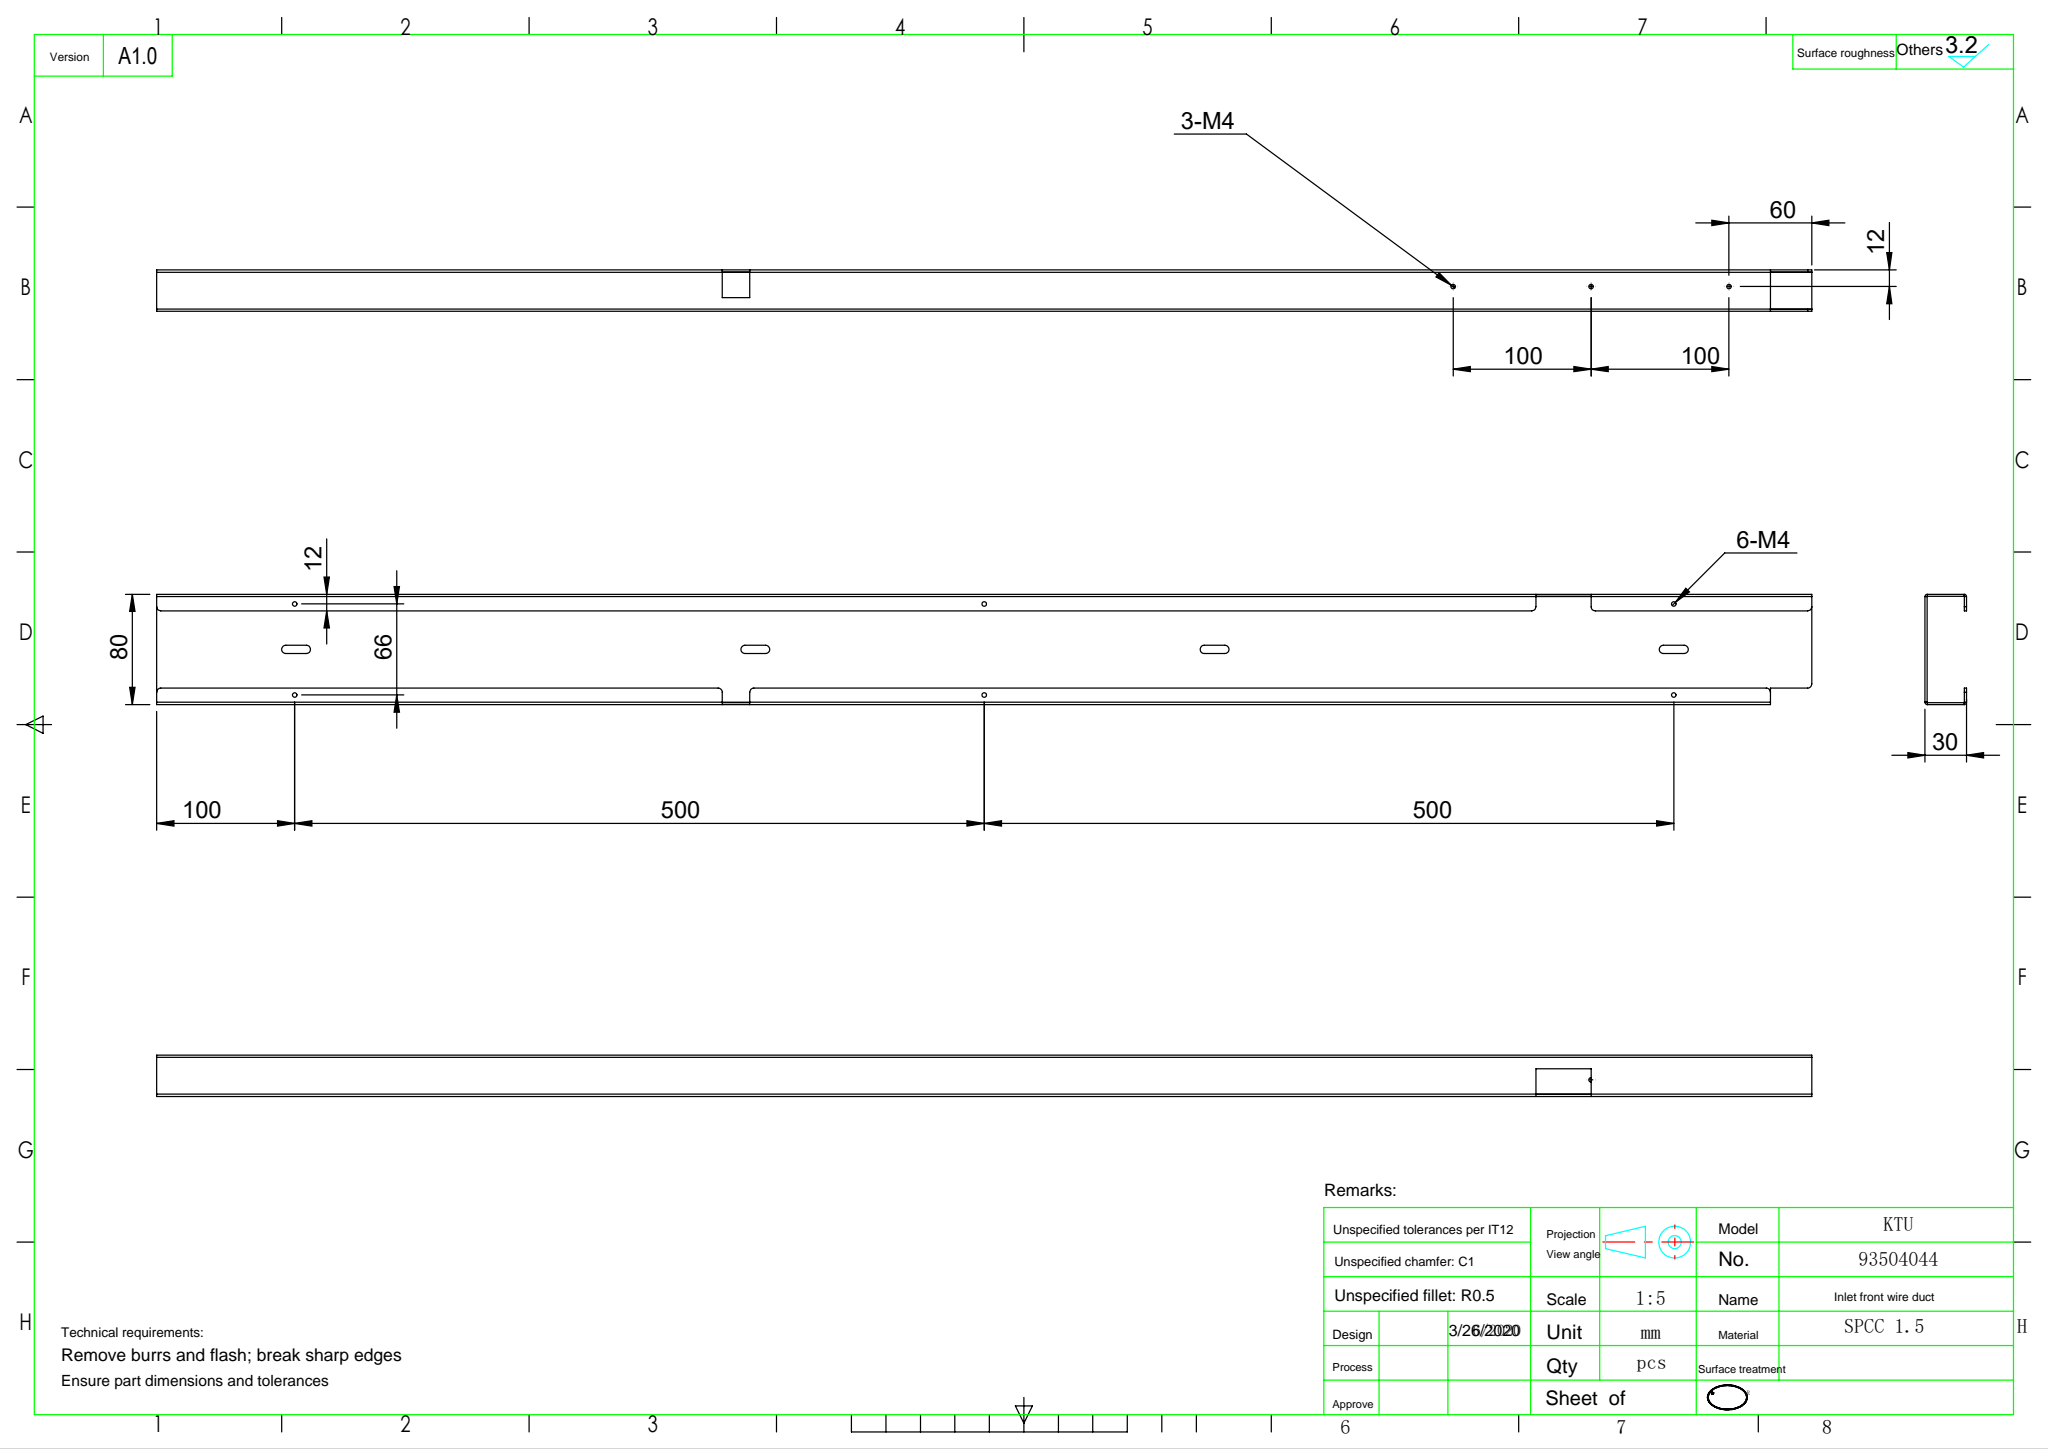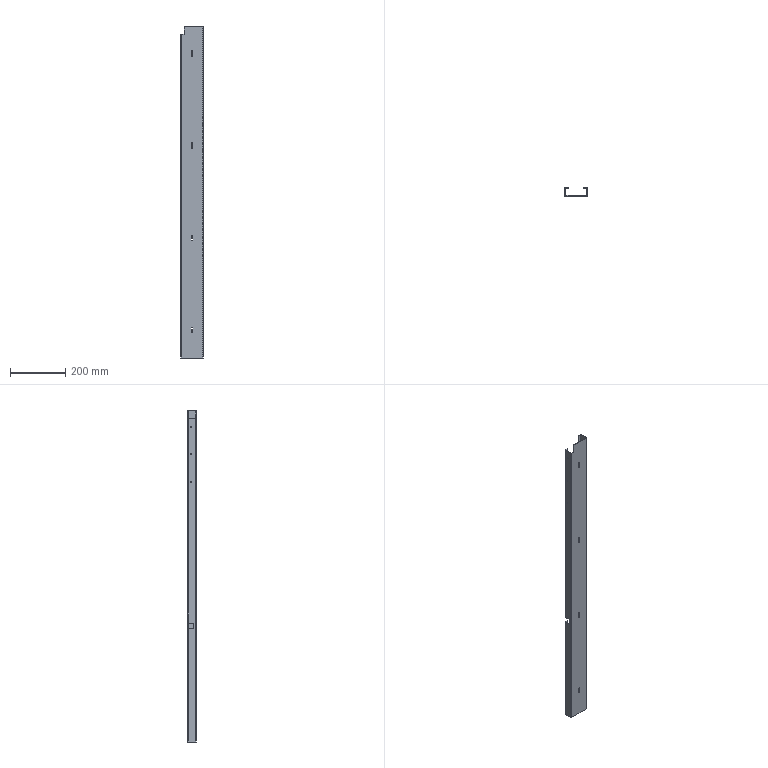Part | SolidWorks | features ICE 3, HoleWzd 2, LPattern 2, Cut 1, Fillet 1, FlatPattern 1, SMBaseFlange 1, SheetMetal 1 | 1 solid | 99 faces | box 80 x 30 x 1200 mm | volume 275646 mm3 | cylinder 51 | plane 48 | commonest cylinder face diameters 6 x21 3.3 x18 0.4 x6 3.4 x6